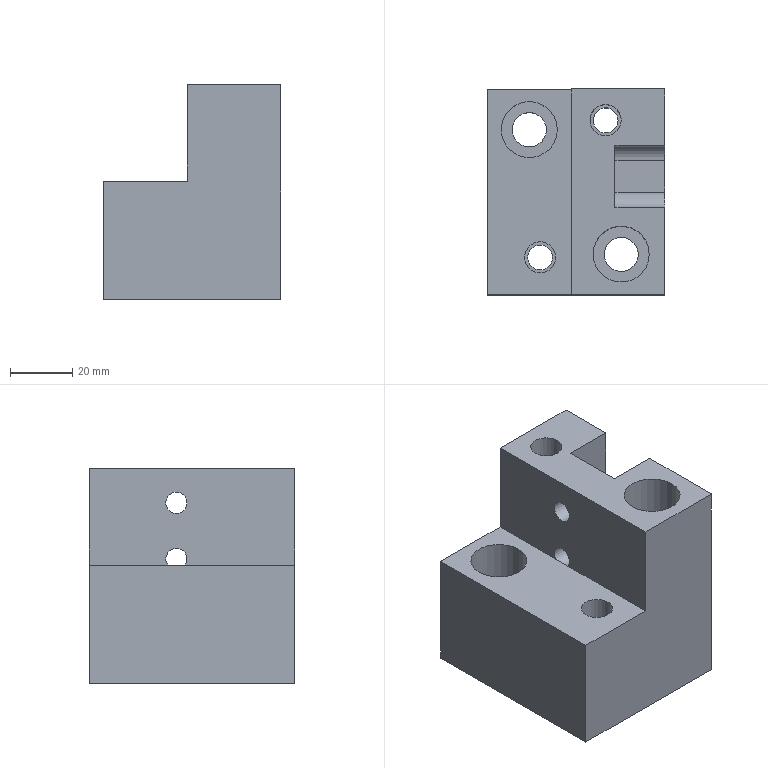Part | STEP file | gslz 2016.10.28-13_id362_x_t | 1 solid | 29 faces | box 57 x 66 x 69 mm | volume 163987 mm3 | plane 17 | cylinder 12 | commonest cylinder face diameters 10 x4 6.8 x2 8 x2 11 x2 18 x2